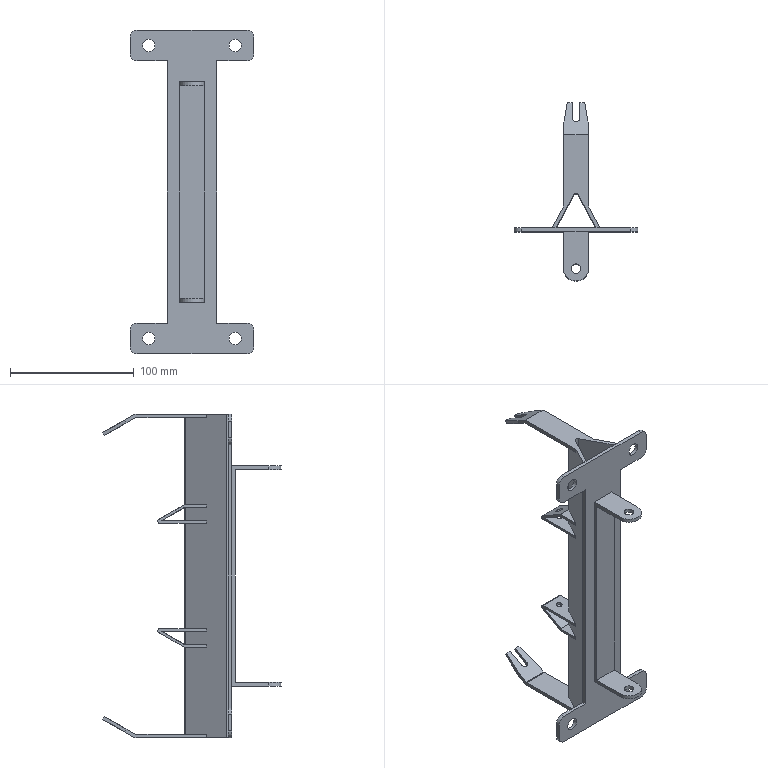Part | STEP file | Frame Idler_1 | 1 solid | 101 faces | box 100 x 144.231 x 262 mm | volume 126128 mm3 | plane 67 | cylinder 34 | commonest cylinder face diameters 12 x8 2 x5 6 x4 10 x4 4 x3 3.353 x2